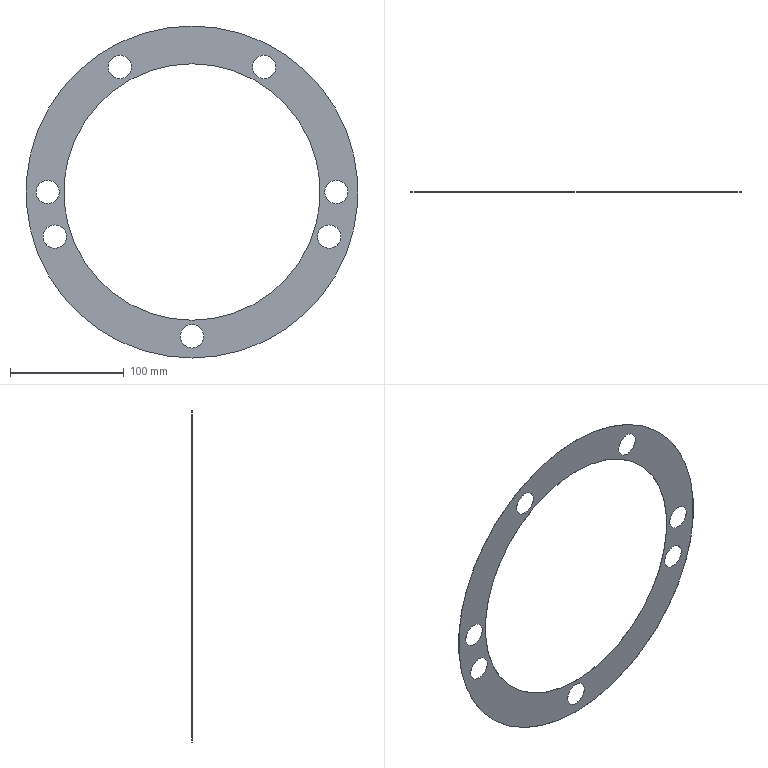Part | SolidWorks | features HoleWzd 2, Extrusion 1, MirrorPattern 1 | 1 solid | 20 faces | box 292.1 x 0.1778 x 292.1 mm | volume 4394 mm3 | cylinder 18 | plane 2 | commonest cylinder face diameters 20.637 x14 225.552 x2 292.1 x2
STEP:
#1=CARTESIAN_POINT('',(-63.5,0.1778,120.301));
#2=VERTEX_POINT('',#1);
#3=CARTESIAN_POINT('',(-63.5,0.1778,99.663));
#4=VERTEX_POINT('',#3);
#5=CARTESIAN_POINT('',(-63.5,0.1778,109.982));
#6=DIRECTION('',(0.,-1.,0.));
#7=DIRECTION('',(0.,0.,-1.));
#8=AXIS2_PLACEMENT_3D('',#5,#6,#7);
#9=CIRCLE('',#8,10.319);
#10=EDGE_CURVE('',#2,#4,#9,.T.);
#11=ORIENTED_EDGE('',*,*,#10,.F.);
#12=CARTESIAN_POINT('',(-63.5,0.,120.301));
#13=VERTEX_POINT('',#12);
#14=CARTESIAN_POINT('',(-63.5,0.,120.301));
#15=DIRECTION('',(0.,-1.,0.));
#16=VECTOR('',#15,1000.);
#17=LINE('',#14,#16);
#18=EDGE_CURVE('',#2,#13,#17,.T.);
#19=ORIENTED_EDGE('',*,*,#18,.T.);
#20=CARTESIAN_POINT('',(-63.5,0.,99.663));
#21=VERTEX_POINT('',#20);
#22=CARTESIAN_POINT('',(-63.5,0.,109.982));
#23=DIRECTION('',(0.,-1.,0.));
#24=DIRECTION('',(0.,0.,-1.));
#25=AXIS2_PLACEMENT_3D('',#22,#23,#24);
#26=CIRCLE('',#25,10.319);
#27=EDGE_CURVE('',#13,#21,#26,.T.);
#28=ORIENTED_EDGE('',*,*,#27,.T.);
#29=CARTESIAN_POINT('',(-63.5,0.,99.663));
#30=DIRECTION('',(0.,-1.,0.));
#31=VECTOR('',#30,1000.);
#32=LINE('',#29,#31);
#33=EDGE_CURVE('',#4,#21,#32,.T.);
#34=ORIENTED_EDGE('',*,*,#33,.F.);
#35=EDGE_LOOP('',(#11,#19,#28,#34));
#36=FACE_OUTER_BOUND('',#35,.T.);
#37=CARTESIAN_POINT('',(-63.5,0.,109.982));
#38=DIRECTION('',(0.,-1.,0.));
#39=DIRECTION('',(0.,0.,-1.));
#40=AXIS2_PLACEMENT_3D('',#37,#38,#39);
#41=CYLINDRICAL_SURFACE('',#40,10.319);
#42=ADVANCED_FACE('',(#36),#41,.F.);
#43=CARTESIAN_POINT('',(-120.77,0.1778,-28.924));
#44=VERTEX_POINT('',#43);
#45=CARTESIAN_POINT('',(-120.77,0.1778,-49.562));
#46=VERTEX_POINT('',#45);
#47=CARTESIAN_POINT('',(-120.77,0.1778,-39.243));
#48=DIRECTION('',(0.,-1.,0.));
#49=DIRECTION('',(0.,0.,-1.));
#50=AXIS2_PLACEMENT_3D('',#47,#48,#49);
#51=CIRCLE('',#50,10.319);
#52=EDGE_CURVE('',#44,#46,#51,.T.);
#53=ORIENTED_EDGE('',*,*,#52,.F.);
#54=CARTESIAN_POINT('',(-120.77,0.,-28.924));
#55=VERTEX_POINT('',#54);
#56=CARTESIAN_POINT('',(-120.77,0.,-28.924));
#57=DIRECTION('',(0.,-1.,0.));
#58=VECTOR('',#57,1000.);
#59=LINE('',#56,#58);
#60=EDGE_CURVE('',#44,#55,#59,.T.);
#61=ORIENTED_EDGE('',*,*,#60,.T.);
#62=CARTESIAN_POINT('',(-120.77,0.,-49.562));
#63=VERTEX_POINT('',#62);
#64=CARTESIAN_POINT('',(-120.77,0.,-39.243));
#65=DIRECTION('',(0.,-1.,0.));
#66=DIRECTION('',(0.,0.,-1.));
#67=AXIS2_PLACEMENT_3D('',#64,#65,#66);
#68=CIRCLE('',#67,10.319);
#69=EDGE_CURVE('',#55,#63,#68,.T.);
#70=ORIENTED_EDGE('',*,*,#69,.T.);
#71=CARTESIAN_POINT('',(-120.77,0.,-49.562));
#72=DIRECTION('',(0.,-1.,0.));
#73=VECTOR('',#72,1000.);
#74=LINE('',#71,#73);
#75=EDGE_CURVE('',#46,#63,#74,.T.);
#76=ORIENTED_EDGE('',*,*,#75,.F.);
#77=EDGE_LOOP('',(#53,#61,#70,#76));
#78=FACE_OUTER_BOUND('',#77,.T.);
#79=CARTESIAN_POINT('',(-120.77,0.,-39.243));
#80=DIRECTION('',(0.,-1.,0.));
#81=DIRECTION('',(0.,0.,-1.));
#82=AXIS2_PLACEMENT_3D('',#79,#80,#81);
#83=CYLINDRICAL_SURFACE('',#82,10.319);
#84=ADVANCED_FACE('',(#78),#83,.F.);
#85=CARTESIAN_POINT('',(-127.,0.1778,10.319));
#86=VERTEX_POINT('',#85);
#87=CARTESIAN_POINT('',(-127.,0.1778,-10.319));
#88=VERTEX_POINT('',#87);
#89=CARTESIAN_POINT('',(-127.,0.1778,0.));
#90=DIRECTION('',(0.,-1.,0.));
#91=DIRECTION('',(0.,0.,-1.));
#92=AXIS2_PLACEMENT_3D('',#89,#90,#91);
#93=CIRCLE('',#92,10.319);
#94=EDGE_CURVE('',#86,#88,#93,.T.);
#95=ORIENTED_EDGE('',*,*,#94,.F.);
#96=CARTESIAN_POINT('',(-127.,0.,10.319));
#97=VERTEX_POINT('',#96);
#98=CARTESIAN_POINT('',(-127.,0.,10.319));
#99=DIRECTION('',(0.,-1.,0.));
#100=VECTOR('',#99,1000.);
#101=LINE('',#98,#100);
#102=EDGE_CURVE('',#86,#97,#101,.T.);
#103=ORIENTED_EDGE('',*,*,#102,.T.);
#104=CARTESIAN_POINT('',(-127.,0.,-10.319));
#105=VERTEX_POINT('',#104);
#106=CARTESIAN_POINT('',(-127.,0.,0.));
#107=DIRECTION('',(0.,-1.,0.));
#108=DIRECTION('',(0.,0.,-1.));
#109=AXIS2_PLACEMENT_3D('',#106,#107,#108);
#110=CIRCLE('',#109,10.319);
#111=EDGE_CURVE('',#97,#105,#110,.T.);
#112=ORIENTED_EDGE('',*,*,#111,.T.);
#113=CARTESIAN_POINT('',(-127.,0.,-10.319));
#114=DIRECTION('',(0.,-1.,0.));
#115=VECTOR('',#114,1000.);
#116=LINE('',#113,#115);
#117=EDGE_CURVE('',#88,#105,#116,.T.);
#118=ORIENTED_EDGE('',*,*,#117,.F.);
#119=EDGE_LOOP('',(#95,#103,#112,#118));
#120=FACE_OUTER_BOUND('',#119,.T.);
#121=CARTESIAN_POINT('',(-127.,0.,0.));
#122=DIRECTION('',(0.,-1.,0.));
#123=DIRECTION('',(0.,0.,-1.));
#124=AXIS2_PLACEMENT_3D('',#121,#122,#123);
#125=CYLINDRICAL_SURFACE('',#124,10.319);
#126=ADVANCED_FACE('',(#120),#125,.F.);
#127=CARTESIAN_POINT('',(63.5,0.1778,120.301));
#128=VERTEX_POINT('',#127);
#129=CARTESIAN_POINT('',(63.5,0.1778,99.663));
#130=VERTEX_POINT('',#129);
#131=CARTESIAN_POINT('',(63.5,0.1778,109.982));
#132=DIRECTION('',(0.,-1.,0.));
#133=DIRECTION('',(0.,0.,-1.));
#134=AXIS2_PLACEMENT_3D('',#131,#132,#133);
#135=CIRCLE('',#134,10.319);
#136=EDGE_CURVE('',#128,#130,#135,.T.);
#137=ORIENTED_EDGE('',*,*,#136,.F.);
#138=CARTESIAN_POINT('',(63.5,0.,120.301));
#139=VERTEX_POINT('',#138);
#140=CARTESIAN_POINT('',(63.5,0.,120.301));
#141=DIRECTION('',(0.,-1.,0.));
#142=VECTOR('',#141,1000.);
#143=LINE('',#140,#142);
#144=EDGE_CURVE('',#128,#139,#143,.T.);
#145=ORIENTED_EDGE('',*,*,#144,.T.);
#146=CARTESIAN_POINT('',(63.5,0.,99.663));
#147=VERTEX_POINT('',#146);
#148=CARTESIAN_POINT('',(63.5,0.,109.982));
#149=DIRECTION('',(0.,-1.,0.));
#150=DIRECTION('',(0.,0.,-1.));
#151=AXIS2_PLACEMENT_3D('',#148,#149,#150);
#152=CIRCLE('',#151,10.319);
#153=EDGE_CURVE('',#139,#147,#152,.T.);
#154=ORIENTED_EDGE('',*,*,#153,.T.);
#155=CARTESIAN_POINT('',(63.5,0.,99.663));
#156=DIRECTION('',(0.,-1.,0.));
#157=VECTOR('',#156,1000.);
#158=LINE('',#155,#157);
#159=EDGE_CURVE('',#130,#147,#158,.T.);
#160=ORIENTED_EDGE('',*,*,#159,.F.);
#161=EDGE_LOOP('',(#137,#145,#154,#160));
#162=FACE_OUTER_BOUND('',#161,.T.);
#163=CARTESIAN_POINT('',(63.5,0.,109.982));
#164=DIRECTION('',(0.,-1.,0.));
#165=DIRECTION('',(0.,0.,-1.));
#166=AXIS2_PLACEMENT_3D('',#163,#164,#165);
#167=CYLINDRICAL_SURFACE('',#166,10.319);
#168=ADVANCED_FACE('',(#162),#167,.F.);
#169=CARTESIAN_POINT('',(120.77,0.1778,-28.924));
#170=VERTEX_POINT('',#169);
#171=CARTESIAN_POINT('',(120.77,0.1778,-49.562));
#172=VERTEX_POINT('',#171);
#173=CARTESIAN_POINT('',(120.77,0.1778,-39.243));
#174=DIRECTION('',(0.,-1.,0.));
#175=DIRECTION('',(0.,0.,-1.));
#176=AXIS2_PLACEMENT_3D('',#173,#174,#175);
#177=CIRCLE('',#176,10.319);
#178=EDGE_CURVE('',#170,#172,#177,.T.);
#179=ORIENTED_EDGE('',*,*,#178,.F.);
#180=CARTESIAN_POINT('',(120.77,0.,-28.924));
#181=VERTEX_POINT('',#180);
#182=CARTESIAN_POINT('',(120.77,0.,-28.924));
#183=DIRECTION('',(0.,-1.,0.));
#184=VECTOR('',#183,1000.);
#185=LINE('',#182,#184);
#186=EDGE_CURVE('',#170,#181,#185,.T.);
#187=ORIENTED_EDGE('',*,*,#186,.T.);
#188=CARTESIAN_POINT('',(120.77,0.,-49.562));
#189=VERTEX_POINT('',#188);
#190=CARTESIAN_POINT('',(120.77,0.,-39.243));
#191=DIRECTION('',(0.,-1.,0.));
#192=DIRECTION('',(0.,0.,-1.));
#193=AXIS2_PLACEMENT_3D('',#190,#191,#192);
#194=CIRCLE('',#193,10.319);
#195=EDGE_CURVE('',#181,#189,#194,.T.);
#196=ORIENTED_EDGE('',*,*,#195,.T.);
#197=CARTESIAN_POINT('',(120.77,0.,-49.562));
#198=DIRECTION('',(0.,-1.,0.));
#199=VECTOR('',#198,1000.);
#200=LINE('',#197,#199);
#201=EDGE_CURVE('',#172,#189,#200,.T.);
#202=ORIENTED_EDGE('',*,*,#201,.F.);
#203=EDGE_LOOP('',(#179,#187,#196,#202));
#204=FACE_OUTER_BOUND('',#203,.T.);
#205=CARTESIAN_POINT('',(120.77,0.,-39.243));
#206=DIRECTION('',(0.,-1.,0.));
#207=DIRECTION('',(0.,0.,-1.));
#208=AXIS2_PLACEMENT_3D('',#205,#206,#207);
#209=CYLINDRICAL_SURFACE('',#208,10.319);
#210=ADVANCED_FACE('',(#204),#209,.F.);
#211=CARTESIAN_POINT('',(127.,0.1778,10.319));
#212=VERTEX_POINT('',#211);
#213=CARTESIAN_POINT('',(127.,0.1778,-10.319));
#214=VERTEX_POINT('',#213);
#215=CARTESIAN_POINT('',(127.,0.1778,0.));
#216=DIRECTION('',(0.,-1.,0.));
#217=DIRECTION('',(0.,0.,-1.));
#218=AXIS2_PLACEMENT_3D('',#215,#216,#217);
#219=CIRCLE('',#218,10.319);
#220=EDGE_CURVE('',#212,#214,#219,.T.);
#221=ORIENTED_EDGE('',*,*,#220,.F.);
#222=CARTESIAN_POINT('',(127.,0.,10.319));
#223=VERTEX_POINT('',#222);
#224=CARTESIAN_POINT('',(127.,0.,10.319));
#225=DIRECTION('',(0.,-1.,0.));
#226=VECTOR('',#225,1000.);
#227=LINE('',#224,#226);
#228=EDGE_CURVE('',#212,#223,#227,.T.);
#229=ORIENTED_EDGE('',*,*,#228,.T.);
#230=CARTESIAN_POINT('',(127.,0.,-10.319));
#231=VERTEX_POINT('',#230);
#232=CARTESIAN_POINT('',(127.,0.,0.));
#233=DIRECTION('',(0.,-1.,0.));
#234=DIRECTION('',(0.,0.,-1.));
#235=AXIS2_PLACEMENT_3D('',#232,#233,#234);
#236=CIRCLE('',#235,10.319);
#237=EDGE_CURVE('',#223,#231,#236,.T.);
#238=ORIENTED_EDGE('',*,*,#237,.T.);
#239=CARTESIAN_POINT('',(127.,0.,-10.319));
#240=DIRECTION('',(0.,-1.,0.));
#241=VECTOR('',#240,1000.);
#242=LINE('',#239,#241);
#243=EDGE_CURVE('',#214,#231,#242,.T.);
#244=ORIENTED_EDGE('',*,*,#243,.F.);
#245=EDGE_LOOP('',(#221,#229,#238,#244));
#246=FACE_OUTER_BOUND('',#245,.T.);
#247=CARTESIAN_POINT('',(127.,0.,0.));
#248=DIRECTION('',(0.,-1.,0.));
#249=DIRECTION('',(0.,0.,-1.));
#250=AXIS2_PLACEMENT_3D('',#247,#248,#249);
#251=CYLINDRICAL_SURFACE('',#250,10.319);
#252=ADVANCED_FACE('',(#246),#251,.F.);
#253=CARTESIAN_POINT('',(0.,0.,-137.319));
#254=VERTEX_POINT('',#253);
#255=CARTESIAN_POINT('',(0.,0.,-116.681));
#256=VERTEX_POINT('',#255);
#257=CARTESIAN_POINT('',(0.,0.,-127.));
#258=DIRECTION('',(0.,1.,0.));
#259=DIRECTION('',(0.,0.,1.));
#260=AXIS2_PLACEMENT_3D('',#257,#258,#259);
#261=CIRCLE('',#260,10.319);
#262=EDGE_CURVE('',#254,#256,#261,.T.);
#263=ORIENTED_EDGE('',*,*,#262,.F.);
#264=CARTESIAN_POINT('',(0.,0.1778,-137.319));
#265=VERTEX_POINT('',#264);
#266=CARTESIAN_POINT('',(0.,0.1778,-137.319));
#267=DIRECTION('',(0.,1.,0.));
#268=VECTOR('',#267,1000.);
#269=LINE('',#266,#268);
#270=EDGE_CURVE('',#254,#265,#269,.T.);
#271=ORIENTED_EDGE('',*,*,#270,.T.);
#272=CARTESIAN_POINT('',(0.,0.1778,-116.681));
#273=VERTEX_POINT('',#272);
#274=CARTESIAN_POINT('',(0.,0.1778,-127.));
#275=DIRECTION('',(0.,1.,0.));
#276=DIRECTION('',(0.,0.,1.));
#277=AXIS2_PLACEMENT_3D('',#274,#275,#276);
#278=CIRCLE('',#277,10.319);
#279=EDGE_CURVE('',#265,#273,#278,.T.);
#280=ORIENTED_EDGE('',*,*,#279,.T.);
#281=CARTESIAN_POINT('',(0.,0.1778,-116.681));
#282=DIRECTION('',(0.,1.,0.));
#283=VECTOR('',#282,1000.);
#284=LINE('',#281,#283);
#285=EDGE_CURVE('',#256,#273,#284,.T.);
#286=ORIENTED_EDGE('',*,*,#285,.F.);
#287=EDGE_LOOP('',(#263,#271,#280,#286));
#288=FACE_OUTER_BOUND('',#287,.T.);
#289=CARTESIAN_POINT('',(0.,0.1778,-127.));
#290=DIRECTION('',(0.,1.,0.));
#291=DIRECTION('',(0.,0.,1.));
#292=AXIS2_PLACEMENT_3D('',#289,#290,#291);
#293=CYLINDRICAL_SURFACE('',#292,10.319);
#294=ADVANCED_FACE('',(#288),#293,.F.);
#295=CARTESIAN_POINT('',(0.,0.1778,-112.776));
#296=VERTEX_POINT('',#295);
#297=CARTESIAN_POINT('',(0.,0.1778,112.776));
#298=VERTEX_POINT('',#297);
#299=CARTESIAN_POINT('',(0.,0.1778,0.));
#300=DIRECTION('',(0.,1.,0.));
#301=DIRECTION('',(0.,0.,1.));
#302=AXIS2_PLACEMENT_3D('',#299,#300,#301);
#303=CIRCLE('',#302,112.776);
#304=EDGE_CURVE('',#296,#298,#303,.T.);
#305=ORIENTED_EDGE('',*,*,#304,.T.);
#306=CARTESIAN_POINT('',(0.,0.,112.776));
#307=VERTEX_POINT('',#306);
#308=CARTESIAN_POINT('',(0.,0.1778,112.776));
#309=DIRECTION('',(0.,-1.,0.));
#310=VECTOR('',#309,1000.);
#311=LINE('',#308,#310);
#312=EDGE_CURVE('',#298,#307,#311,.T.);
#313=ORIENTED_EDGE('',*,*,#312,.T.);
#314=CARTESIAN_POINT('',(0.,0.,-112.776));
#315=VERTEX_POINT('',#314);
#316=CARTESIAN_POINT('',(0.,0.,0.));
#317=DIRECTION('',(0.,1.,0.));
#318=DIRECTION('',(0.,0.,1.));
#319=AXIS2_PLACEMENT_3D('',#316,#317,#318);
#320=CIRCLE('',#319,112.776);
#321=EDGE_CURVE('',#315,#307,#320,.T.);
#322=ORIENTED_EDGE('',*,*,#321,.F.);
#323=CARTESIAN_POINT('',(0.,0.1778,-112.776));
#324=DIRECTION('',(0.,-1.,0.));
#325=VECTOR('',#324,1000.);
#326=LINE('',#323,#325);
#327=EDGE_CURVE('',#296,#315,#326,.T.);
#328=ORIENTED_EDGE('',*,*,#327,.F.);
#329=EDGE_LOOP('',(#305,#313,#322,#328));
#330=FACE_OUTER_BOUND('',#329,.T.);
#331=CARTESIAN_POINT('',(0.,0.1778,0.));
#332=DIRECTION('',(0.,-1.,0.));
#333=DIRECTION('',(0.,0.,-1.));
#334=AXIS2_PLACEMENT_3D('',#331,#332,#333);
#335=CYLINDRICAL_SURFACE('',#334,112.776);
#336=ADVANCED_FACE('',(#330),#335,.F.);
#337=CARTESIAN_POINT('',(0.,0.1778,146.05));
#338=VERTEX_POINT('',#337);
#339=CARTESIAN_POINT('',(0.,0.1778,-146.05));
#340=VERTEX_POINT('',#339);
#341=CARTESIAN_POINT('',(0.,0.1778,0.));
#342=DIRECTION('',(0.,1.,0.));
#343=DIRECTION('',(0.,0.,1.));
#344=AXIS2_PLACEMENT_3D('',#341,#342,#343);
#345=CIRCLE('',#344,146.05);
#346=EDGE_CURVE('',#338,#340,#345,.T.);
#347=ORIENTED_EDGE('',*,*,#346,.F.);
#348=CARTESIAN_POINT('',(0.,0.,146.05));
#349=VERTEX_POINT('',#348);
#350=CARTESIAN_POINT('',(0.,0.1778,146.05));
#351=DIRECTION('',(0.,-1.,0.));
#352=VECTOR('',#351,1000.);
#353=LINE('',#350,#352);
#354=EDGE_CURVE('',#338,#349,#353,.T.);
#355=ORIENTED_EDGE('',*,*,#354,.T.);
#356=CARTESIAN_POINT('',(0.,0.,-146.05));
#357=VERTEX_POINT('',#356);
#358=CARTESIAN_POINT('',(0.,0.,0.));
#359=DIRECTION('',(0.,1.,0.));
#360=DIRECTION('',(0.,0.,1.));
#361=AXIS2_PLACEMENT_3D('',#358,#359,#360);
#362=CIRCLE('',#361,146.05);
#363=EDGE_CURVE('',#349,#357,#362,.T.);
#364=ORIENTED_EDGE('',*,*,#363,.T.);
#365=CARTESIAN_POINT('',(0.,0.1778,-146.05));
#366=DIRECTION('',(0.,-1.,0.));
#367=VECTOR('',#366,1000.);
#368=LINE('',#365,#367);
#369=EDGE_CURVE('',#340,#357,#368,.T.);
#370=ORIENTED_EDGE('',*,*,#369,.F.);
#371=EDGE_LOOP('',(#347,#355,#364,#370));
#372=FACE_OUTER_BOUND('',#371,.T.);
#373=CARTESIAN_POINT('',(0.,0.1778,0.));
#374=DIRECTION('',(0.,-1.,0.));
#375=DIRECTION('',(0.,0.,-1.));
#376=AXIS2_PLACEMENT_3D('',#373,#374,#375);
#377=CYLINDRICAL_SURFACE('',#376,146.05);
#378=ADVANCED_FACE('',(#372),#377,.T.);
#379=CARTESIAN_POINT('',(-120.77,0.,-39.243));
#380=DIRECTION('',(0.,-1.,0.));
#381=DIRECTION('',(0.,0.,-1.));
#382=AXIS2_PLACEMENT_3D('',#379,#380,#381);
#383=CIRCLE('',#382,10.319);
#384=EDGE_CURVE('',#63,#55,#383,.T.);
#385=ORIENTED_EDGE('',*,*,#384,.F.);
#386=ORIENTED_EDGE('',*,*,#69,.F.);
#387=EDGE_LOOP('',(#385,#386));
#388=FACE_BOUND('',#387,.T.);
#389=ORIENTED_EDGE('',*,*,#321,.T.);
#390=CARTESIAN_POINT('',(0.,0.,0.));
#391=DIRECTION('',(0.,1.,0.));
#392=DIRECTION('',(0.,0.,1.));
#393=AXIS2_PLACEMENT_3D('',#390,#391,#392);
#394=CIRCLE('',#393,112.776);
#395=EDGE_CURVE('',#307,#315,#394,.T.);
#396=ORIENTED_EDGE('',*,*,#395,.T.);
#397=EDGE_LOOP('',(#389,#396));
#398=FACE_BOUND('',#397,.T.);
#399=CARTESIAN_POINT('',(0.,0.,0.));
#400=DIRECTION('',(0.,1.,0.));
#401=DIRECTION('',(0.,0.,1.));
#402=AXIS2_PLACEMENT_3D('',#399,#400,#401);
#403=CIRCLE('',#402,146.05);
#404=EDGE_CURVE('',#357,#349,#403,.T.);
#405=ORIENTED_EDGE('',*,*,#404,.F.);
#406=ORIENTED_EDGE('',*,*,#363,.F.);
#407=EDGE_LOOP('',(#405,#406));
#408=FACE_OUTER_BOUND('',#407,.T.);
#409=CARTESIAN_POINT('',(0.,0.,-127.));
#410=DIRECTION('',(0.,1.,0.));
#411=DIRECTION('',(0.,0.,1.));
#412=AXIS2_PLACEMENT_3D('',#409,#410,#411);
#413=CIRCLE('',#412,10.319);
#414=EDGE_CURVE('',#256,#254,#413,.T.);
#415=ORIENTED_EDGE('',*,*,#414,.T.);
#416=ORIENTED_EDGE('',*,*,#262,.T.);
#417=EDGE_LOOP('',(#415,#416));
#418=FACE_BOUND('',#417,.T.);
#419=CARTESIAN_POINT('',(127.,0.,0.));
#420=DIRECTION('',(0.,-1.,0.));
#421=DIRECTION('',(0.,0.,-1.));
#422=AXIS2_PLACEMENT_3D('',#419,#420,#421);
#423=CIRCLE('',#422,10.319);
#424=EDGE_CURVE('',#231,#223,#423,.T.);
#425=ORIENTED_EDGE('',*,*,#424,.F.);
#426=ORIENTED_EDGE('',*,*,#237,.F.);
#427=EDGE_LOOP('',(#425,#426));
#428=FACE_BOUND('',#427,.T.);
#429=CARTESIAN_POINT('',(120.77,0.,-39.243));
#430=DIRECTION('',(0.,-1.,0.));
#431=DIRECTION('',(0.,0.,-1.));
#432=AXIS2_PLACEMENT_3D('',#429,#430,#431);
#433=CIRCLE('',#432,10.319);
#434=EDGE_CURVE('',#189,#181,#433,.T.);
#435=ORIENTED_EDGE('',*,*,#434,.F.);
#436=ORIENTED_EDGE('',*,*,#195,.F.);
#437=EDGE_LOOP('',(#435,#436));
#438=FACE_BOUND('',#437,.T.);
#439=CARTESIAN_POINT('',(63.5,0.,109.982));
#440=DIRECTION('',(0.,-1.,0.));
#441=DIRECTION('',(0.,0.,-1.));
#442=AXIS2_PLACEMENT_3D('',#439,#440,#441);
#443=CIRCLE('',#442,10.319);
#444=EDGE_CURVE('',#147,#139,#443,.T.);
#445=ORIENTED_EDGE('',*,*,#444,.F.);
#446=ORIENTED_EDGE('',*,*,#153,.F.);
#447=EDGE_LOOP('',(#445,#446));
#448=FACE_BOUND('',#447,.T.);
#449=CARTESIAN_POINT('',(-127.,0.,0.));
#450=DIRECTION('',(0.,-1.,0.));
#451=DIRECTION('',(0.,0.,-1.));
#452=AXIS2_PLACEMENT_3D('',#449,#450,#451);
#453=CIRCLE('',#452,10.319);
#454=EDGE_CURVE('',#105,#97,#453,.T.);
#455=ORIENTED_EDGE('',*,*,#454,.F.);
#456=ORIENTED_EDGE('',*,*,#111,.F.);
#457=EDGE_LOOP('',(#455,#456));
#458=FACE_BOUND('',#457,.T.);
#459=CARTESIAN_POINT('',(-63.5,0.,109.982));
#460=DIRECTION('',(0.,-1.,0.));
#461=DIRECTION('',(0.,0.,-1.));
#462=AXIS2_PLACEMENT_3D('',#459,#460,#461);
#463=CIRCLE('',#462,10.319);
#464=EDGE_CURVE('',#21,#13,#463,.T.);
#465=ORIENTED_EDGE('',*,*,#464,.F.);
#466=ORIENTED_EDGE('',*,*,#27,.F.);
#467=EDGE_LOOP('',(#465,#466));
#468=FACE_BOUND('',#467,.T.);
#469=CARTESIAN_POINT('',(0.,0.,0.));
#470=DIRECTION('',(0.,1.,0.));
#471=DIRECTION('',(0.,0.,1.));
#472=AXIS2_PLACEMENT_3D('',#469,#470,#471);
#473=PLANE('',#472);
#474=ADVANCED_FACE('',(#388,#398,#408,#418,#428,#438,#448,#458,#468),#473,.F.);
#475=CARTESIAN_POINT('',(-120.77,0.1778,-39.243));
#476=DIRECTION('',(0.,-1.,0.));
#477=DIRECTION('',(0.,0.,-1.));
#478=AXIS2_PLACEMENT_3D('',#475,#476,#477);
#479=CIRCLE('',#478,10.319);
#480=EDGE_CURVE('',#46,#44,#479,.T.);
#481=ORIENTED_EDGE('',*,*,#480,.T.);
#482=ORIENTED_EDGE('',*,*,#52,.T.);
#483=EDGE_LOOP('',(#481,#482));
#484=FACE_BOUND('',#483,.T.);
#485=CARTESIAN_POINT('',(-127.,0.1778,0.));
#486=DIRECTION('',(0.,-1.,0.));
#487=DIRECTION('',(0.,0.,-1.));
#488=AXIS2_PLACEMENT_3D('',#485,#486,#487);
#489=CIRCLE('',#488,10.319);
#490=EDGE_CURVE('',#88,#86,#489,.T.);
#491=ORIENTED_EDGE('',*,*,#490,.T.);
#492=ORIENTED_EDGE('',*,*,#94,.T.);
#493=EDGE_LOOP('',(#491,#492));
#494=FACE_BOUND('',#493,.T.);
#495=CARTESIAN_POINT('',(63.5,0.1778,109.982));
#496=DIRECTION('',(0.,-1.,0.));
#497=DIRECTION('',(0.,0.,-1.));
#498=AXIS2_PLACEMENT_3D('',#495,#496,#497);
#499=CIRCLE('',#498,10.319);
#500=EDGE_CURVE('',#130,#128,#499,.T.);
#501=ORIENTED_EDGE('',*,*,#500,.T.);
#502=ORIENTED_EDGE('',*,*,#136,.T.);
#503=EDGE_LOOP('',(#501,#502));
#504=FACE_BOUND('',#503,.T.);
#505=CARTESIAN_POINT('',(120.77,0.1778,-39.243));
#506=DIRECTION('',(0.,-1.,0.));
#507=DIRECTION('',(0.,0.,-1.));
#508=AXIS2_PLACEMENT_3D('',#505,#506,#507);
#509=CIRCLE('',#508,10.319);
#510=EDGE_CURVE('',#172,#170,#509,.T.);
#511=ORIENTED_EDGE('',*,*,#510,.T.);
#512=ORIENTED_EDGE('',*,*,#178,.T.);
#513=EDGE_LOOP('',(#511,#512));
#514=FACE_BOUND('',#513,.T.);
#515=CARTESIAN_POINT('',(127.,0.1778,0.));
#516=DIRECTION('',(0.,-1.,0.));
#517=DIRECTION('',(0.,0.,-1.));
#518=AXIS2_PLACEMENT_3D('',#515,#516,#517);
#519=CIRCLE('',#518,10.319);
#520=EDGE_CURVE('',#214,#212,#519,.T.);
#521=ORIENTED_EDGE('',*,*,#520,.T.);
#522=ORIENTED_EDGE('',*,*,#220,.T.);
#523=EDGE_LOOP('',(#521,#522));
#524=FACE_BOUND('',#523,.T.);
#525=CARTESIAN_POINT('',(0.,0.1778,-127.));
#526=DIRECTION('',(0.,1.,0.));
#527=DIRECTION('',(0.,0.,1.));
#528=AXIS2_PLACEMENT_3D('',#525,#526,#527);
#529=CIRCLE('',#528,10.319);
#530=EDGE_CURVE('',#273,#265,#529,.T.);
#531=ORIENTED_EDGE('',*,*,#530,.F.);
#532=ORIENTED_EDGE('',*,*,#279,.F.);
#533=EDGE_LOOP('',(#531,#532));
#534=FACE_BOUND('',#533,.T.);
#535=CARTESIAN_POINT('',(0.,0.1778,0.));
#536=DIRECTION('',(0.,1.,0.));
#537=DIRECTION('',(0.,0.,1.));
#538=AXIS2_PLACEMENT_3D('',#535,#536,#537);
#539=CIRCLE('',#538,146.05);
#540=EDGE_CURVE('',#340,#338,#539,.T.);
#541=ORIENTED_EDGE('',*,*,#540,.T.);
#542=ORIENTED_EDGE('',*,*,#346,.T.);
#543=EDGE_LOOP('',(#541,#542));
#544=FACE_OUTER_BOUND('',#543,.T.);
#545=ORIENTED_EDGE('',*,*,#304,.F.);
#546=CARTESIAN_POINT('',(0.,0.1778,0.));
#547=DIRECTION('',(0.,1.,0.));
#548=DIRECTION('',(0.,0.,1.));
#549=AXIS2_PLACEMENT_3D('',#546,#547,#548);
#550=CIRCLE('',#549,112.776);
#551=EDGE_CURVE('',#298,#296,#550,.T.);
#552=ORIENTED_EDGE('',*,*,#551,.F.);
#553=EDGE_LOOP('',(#545,#552));
#554=FACE_BOUND('',#553,.T.);
#555=CARTESIAN_POINT('',(-63.5,0.1778,109.982));
#556=DIRECTION('',(0.,-1.,0.));
#557=DIRECTION('',(0.,0.,-1.));
#558=AXIS2_PLACEMENT_3D('',#555,#556,#557);
#559=CIRCLE('',#558,10.319);
#560=EDGE_CURVE('',#4,#2,#559,.T.);
#561=ORIENTED_EDGE('',*,*,#560,.T.);
#562=ORIENTED_EDGE('',*,*,#10,.T.);
#563=EDGE_LOOP('',(#561,#562));
#564=FACE_BOUND('',#563,.T.);
#565=CARTESIAN_POINT('',(0.,0.1778,0.));
#566=DIRECTION('',(0.,1.,0.));
#567=DIRECTION('',(0.,0.,1.));
#568=AXIS2_PLACEMENT_3D('',#565,#566,#567);
#569=PLANE('',#568);
#570=ADVANCED_FACE('',(#484,#494,#504,#514,#524,#534,#544,#554,#564),#569,.T.);
#571=ORIENTED_EDGE('',*,*,#354,.F.);
#572=ORIENTED_EDGE('',*,*,#540,.F.);
#573=ORIENTED_EDGE('',*,*,#369,.T.);
#574=ORIENTED_EDGE('',*,*,#404,.T.);
#575=EDGE_LOOP('',(#571,#572,#573,#574));
#576=FACE_OUTER_BOUND('',#575,.T.);
#577=CARTESIAN_POINT('',(0.,0.1778,0.));
#578=DIRECTION('',(0.,-1.,0.));
#579=DIRECTION('',(0.,0.,-1.));
#580=AXIS2_PLACEMENT_3D('',#577,#578,#579);
#581=CYLINDRICAL_SURFACE('',#580,146.05);
#582=ADVANCED_FACE('',(#576),#581,.T.);
#583=ORIENTED_EDGE('',*,*,#312,.F.);
#584=ORIENTED_EDGE('',*,*,#551,.T.);
#585=ORIENTED_EDGE('',*,*,#327,.T.);
#586=ORIENTED_EDGE('',*,*,#395,.F.);
#587=EDGE_LOOP('',(#583,#584,#585,#586));
#588=FACE_OUTER_BOUND('',#587,.T.);
#589=CARTESIAN_POINT('',(0.,0.1778,0.));
#590=DIRECTION('',(0.,-1.,0.));
#591=DIRECTION('',(0.,0.,-1.));
#592=AXIS2_PLACEMENT_3D('',#589,#590,#591);
#593=CYLINDRICAL_SURFACE('',#592,112.776);
#594=ADVANCED_FACE('',(#588),#593,.F.);
#595=ORIENTED_EDGE('',*,*,#270,.F.);
#596=ORIENTED_EDGE('',*,*,#414,.F.);
#597=ORIENTED_EDGE('',*,*,#285,.T.);
#598=ORIENTED_EDGE('',*,*,#530,.T.);
#599=EDGE_LOOP('',(#595,#596,#597,#598));
#600=FACE_OUTER_BOUND('',#599,.T.);
#601=CARTESIAN_POINT('',(0.,0.1778,-127.));
#602=DIRECTION('',(0.,1.,0.));
#603=DIRECTION('',(0.,0.,1.));
#604=AXIS2_PLACEMENT_3D('',#601,#602,#603);
#605=CYLINDRICAL_SURFACE('',#604,10.319);
#606=ADVANCED_FACE('',(#600),#605,.F.);
#607=ORIENTED_EDGE('',*,*,#228,.F.);
#608=ORIENTED_EDGE('',*,*,#520,.F.);
#609=ORIENTED_EDGE('',*,*,#243,.T.);
#610=ORIENTED_EDGE('',*,*,#424,.T.);
#611=EDGE_LOOP('',(#607,#608,#609,#610));
#612=FACE_OUTER_BOUND('',#611,.T.);
#613=CARTESIAN_POINT('',(127.,0.,0.));
#614=DIRECTION('',(0.,-1.,0.));
#615=DIRECTION('',(0.,0.,-1.));
#616=AXIS2_PLACEMENT_3D('',#613,#614,#615);
#617=CYLINDRICAL_SURFACE('',#616,10.319);
#618=ADVANCED_FACE('',(#612),#617,.F.);
#619=ORIENTED_EDGE('',*,*,#186,.F.);
#620=ORIENTED_EDGE('',*,*,#510,.F.);
#621=ORIENTED_EDGE('',*,*,#201,.T.);
#622=ORIENTED_EDGE('',*,*,#434,.T.);
#623=EDGE_LOOP('',(#619,#620,#621,#622));
#624=FACE_OUTER_BOUND('',#623,.T.);
#625=CARTESIAN_POINT('',(120.77,0.,-39.243));
#626=DIRECTION('',(0.,-1.,0.));
#627=DIRECTION('',(0.,0.,-1.));
#628=AXIS2_PLACEMENT_3D('',#625,#626,#627);
#629=CYLINDRICAL_SURFACE('',#628,10.319);
#630=ADVANCED_FACE('',(#624),#629,.F.);
#631=ORIENTED_EDGE('',*,*,#144,.F.);
#632=ORIENTED_EDGE('',*,*,#500,.F.);
#633=ORIENTED_EDGE('',*,*,#159,.T.);
#634=ORIENTED_EDGE('',*,*,#444,.T.);
#635=EDGE_LOOP('',(#631,#632,#633,#634));
#636=FACE_OUTER_BOUND('',#635,.T.);
#637=CARTESIAN_POINT('',(63.5,0.,109.982));
#638=DIRECTION('',(0.,-1.,0.));
#639=DIRECTION('',(0.,0.,-1.));
#640=AXIS2_PLACEMENT_3D('',#637,#638,#639);
#641=CYLINDRICAL_SURFACE('',#640,10.319);
#642=ADVANCED_FACE('',(#636),#641,.F.);
#643=ORIENTED_EDGE('',*,*,#102,.F.);
#644=ORIENTED_EDGE('',*,*,#490,.F.);
#645=ORIENTED_EDGE('',*,*,#117,.T.);
#646=ORIENTED_EDGE('',*,*,#454,.T.);
#647=EDGE_LOOP('',(#643,#644,#645,#646));
#648=FACE_OUTER_BOUND('',#647,.T.);
#649=CARTESIAN_POINT('',(-127.,0.,0.));
#650=DIRECTION('',(0.,-1.,0.));
#651=DIRECTION('',(0.,0.,-1.));
#652=AXIS2_PLACEMENT_3D('',#649,#650,#651);
#653=CYLINDRICAL_SURFACE('',#652,10.319);
#654=ADVANCED_FACE('',(#648),#653,.F.);
#655=ORIENTED_EDGE('',*,*,#60,.F.);
#656=ORIENTED_EDGE('',*,*,#480,.F.);
#657=ORIENTED_EDGE('',*,*,#75,.T.);
#658=ORIENTED_EDGE('',*,*,#384,.T.);
#659=EDGE_LOOP('',(#655,#656,#657,#658));
#660=FACE_OUTER_BOUND('',#659,.T.);
#661=CARTESIAN_POINT('',(-120.77,0.,-39.243));
#662=DIRECTION('',(0.,-1.,0.));
#663=DIRECTION('',(0.,0.,-1.));
#664=AXIS2_PLACEMENT_3D('',#661,#662,#663);
#665=CYLINDRICAL_SURFACE('',#664,10.319);
#666=ADVANCED_FACE('',(#660),#665,.F.);
#667=ORIENTED_EDGE('',*,*,#18,.F.);
#668=ORIENTED_EDGE('',*,*,#560,.F.);
#669=ORIENTED_EDGE('',*,*,#33,.T.);
#670=ORIENTED_EDGE('',*,*,#464,.T.);
#671=EDGE_LOOP('',(#667,#668,#669,#670));
#672=FACE_OUTER_BOUND('',#671,.T.);
#673=CARTESIAN_POINT('',(-63.5,0.,109.982));
#674=DIRECTION('',(0.,-1.,0.));
#675=DIRECTION('',(0.,0.,-1.));
#676=AXIS2_PLACEMENT_3D('',#673,#674,#675);
#677=CYLINDRICAL_SURFACE('',#676,10.319);
#678=ADVANCED_FACE('',(#672),#677,.F.);
#679=CLOSED_SHELL('',(#42,#84,#126,#168,#210,#252,#294,#336,#378,#474,#570,#582,#594,#606,#618,#630,#642,#654,#666,#678));
#680=MANIFOLD_SOLID_BREP('',#679);
#681=CARTESIAN_POINT('',(0.,0.,0.));
#682=DIRECTION('',(0.,0.,1.));
#683=DIRECTION('',(1.,0.,0.));
#684=AXIS2_PLACEMENT_3D('',#681,#682,#683);
#685=(LENGTH_UNIT()NAMED_UNIT(*)SI_UNIT(.MILLI.,.METRE.));
#686=UNCERTAINTY_MEASURE_WITH_UNIT(LENGTH_MEASURE(0.00001),#685,'','');
#687=(NAMED_UNIT(*)PLANE_ANGLE_UNIT()SI_UNIT($,.RADIAN.));
#688=(NAMED_UNIT(*)SI_UNIT($,.STERADIAN.)SOLID_ANGLE_UNIT());
#689=(GEOMETRIC_REPRESENTATION_CONTEXT(3)GLOBAL_UNCERTAINTY_ASSIGNED_CONTEXT((#686))GLOBAL_UNIT_ASSIGNED_CONTEXT((#685,#687,#688))REPRESENTATION_CONTEXT('',''));
#690=ADVANCED_BREP_SHAPE_REPRESENTATION('',(#680,#684),#689);